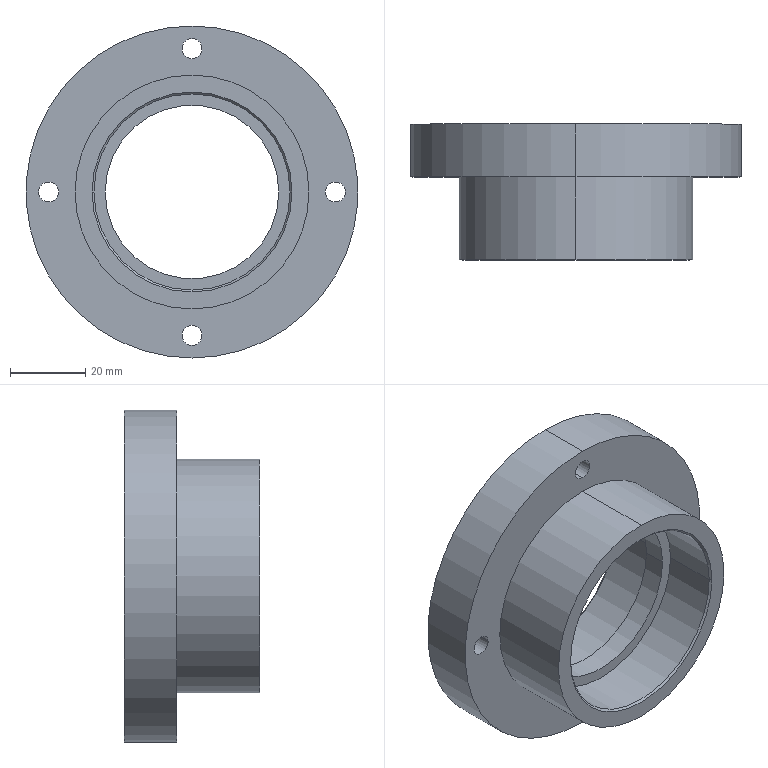Part | NX | 1 solid | 39 faces | box 88 x 36 x 88 mm | volume 75330 mm3 | cylinder 26 | plane 9 | cone 4 | commonest cylinder face diameters 5.3 x8 10 x6 52 x4 9.5 x2 46 x2 62 x2
STEP:
#1=CARTESIAN_POINT('',(0.,-14.,-44.));
#2=VERTEX_POINT('',#1);
#3=CARTESIAN_POINT('',(0.,-14.,44.));
#4=VERTEX_POINT('',#3);
#5=CARTESIAN_POINT('',(0.,-14.,0.));
#6=DIRECTION('',(0.,1.,0.));
#7=DIRECTION('',(0.,0.,1.));
#8=AXIS2_PLACEMENT_3D('',#5,#6,#7);
#9=CIRCLE('',#8,44.);
#10=EDGE_CURVE('',#2,#4,#9,.T.);
#11=ORIENTED_EDGE('',*,*,#10,.F.);
#12=CARTESIAN_POINT('',(0.,-14.,0.));
#13=DIRECTION('',(0.,1.,0.));
#14=DIRECTION('',(0.,0.,1.));
#15=AXIS2_PLACEMENT_3D('',#12,#13,#14);
#16=CIRCLE('',#15,44.);
#17=EDGE_CURVE('',#4,#2,#16,.T.);
#18=ORIENTED_EDGE('',*,*,#17,.F.);
#19=EDGE_LOOP('',(#11,#18));
#20=FACE_BOUND('',#19,.T.);
#21=CARTESIAN_POINT('',(0.,-14.,31.));
#22=VERTEX_POINT('',#21);
#23=CARTESIAN_POINT('',(0.,-14.,-31.));
#24=VERTEX_POINT('',#23);
#25=CARTESIAN_POINT('',(0.,-14.,0.));
#26=DIRECTION('',(0.,-1.,0.));
#27=DIRECTION('',(0.,0.,1.));
#28=AXIS2_PLACEMENT_3D('',#25,#26,#27);
#29=CIRCLE('',#28,31.);
#30=EDGE_CURVE('',#22,#24,#29,.T.);
#31=ORIENTED_EDGE('',*,*,#30,.F.);
#32=CARTESIAN_POINT('',(0.,-14.,0.));
#33=DIRECTION('',(0.,-1.,0.));
#34=DIRECTION('',(0.,0.,1.));
#35=AXIS2_PLACEMENT_3D('',#32,#33,#34);
#36=CIRCLE('',#35,31.);
#37=EDGE_CURVE('',#24,#22,#36,.T.);
#38=ORIENTED_EDGE('',*,*,#37,.F.);
#39=EDGE_LOOP('',(#31,#38));
#40=FACE_BOUND('',#39,.T.);
#41=CARTESIAN_POINT('',(40.65,-14.,0.));
#42=VERTEX_POINT('',#41);
#43=CARTESIAN_POINT('',(35.35,-14.,0.));
#44=VERTEX_POINT('',#43);
#45=CARTESIAN_POINT('',(38.,-14.,0.));
#46=DIRECTION('',(0.,-1.,0.));
#47=DIRECTION('',(1.,0.,0.));
#48=AXIS2_PLACEMENT_3D('',#45,#46,#47);
#49=CIRCLE('',#48,2.65);
#50=EDGE_CURVE('',#42,#44,#49,.T.);
#51=ORIENTED_EDGE('',*,*,#50,.F.);
#52=CARTESIAN_POINT('',(38.,-14.,0.));
#53=DIRECTION('',(0.,-1.,0.));
#54=DIRECTION('',(1.,0.,0.));
#55=AXIS2_PLACEMENT_3D('',#52,#53,#54);
#56=CIRCLE('',#55,2.65);
#57=EDGE_CURVE('',#44,#42,#56,.T.);
#58=ORIENTED_EDGE('',*,*,#57,.F.);
#59=EDGE_LOOP('',(#51,#58));
#60=FACE_BOUND('',#59,.T.);
#61=CARTESIAN_POINT('',(0.,-14.,-35.35));
#62=VERTEX_POINT('',#61);
#63=CARTESIAN_POINT('',(0.,-14.,-40.65));
#64=VERTEX_POINT('',#63);
#65=CARTESIAN_POINT('',(0.,-14.,-38.));
#66=DIRECTION('',(0.,-1.,0.));
#67=DIRECTION('',(0.,0.,-1.));
#68=AXIS2_PLACEMENT_3D('',#65,#66,#67);
#69=CIRCLE('',#68,2.65);
#70=EDGE_CURVE('',#62,#64,#69,.T.);
#71=ORIENTED_EDGE('',*,*,#70,.F.);
#72=CARTESIAN_POINT('',(0.,-14.,-38.));
#73=DIRECTION('',(0.,-1.,0.));
#74=DIRECTION('',(0.,0.,-1.));
#75=AXIS2_PLACEMENT_3D('',#72,#73,#74);
#76=CIRCLE('',#75,2.65);
#77=EDGE_CURVE('',#64,#62,#76,.T.);
#78=ORIENTED_EDGE('',*,*,#77,.F.);
#79=EDGE_LOOP('',(#71,#78));
#80=FACE_BOUND('',#79,.T.);
#81=CARTESIAN_POINT('',(-40.65,-14.,0.));
#82=VERTEX_POINT('',#81);
#83=CARTESIAN_POINT('',(-35.35,-14.,0.));
#84=VERTEX_POINT('',#83);
#85=CARTESIAN_POINT('',(-38.,-14.,0.));
#86=DIRECTION('',(0.,-1.,0.));
#87=DIRECTION('',(-1.,0.,0.));
#88=AXIS2_PLACEMENT_3D('',#85,#86,#87);
#89=CIRCLE('',#88,2.65);
#90=EDGE_CURVE('',#82,#84,#89,.T.);
#91=ORIENTED_EDGE('',*,*,#90,.F.);
#92=CARTESIAN_POINT('',(-38.,-14.,0.));
#93=DIRECTION('',(0.,-1.,0.));
#94=DIRECTION('',(-1.,0.,0.));
#95=AXIS2_PLACEMENT_3D('',#92,#93,#94);
#96=CIRCLE('',#95,2.65);
#97=EDGE_CURVE('',#84,#82,#96,.T.);
#98=ORIENTED_EDGE('',*,*,#97,.F.);
#99=EDGE_LOOP('',(#91,#98));
#100=FACE_BOUND('',#99,.T.);
#101=CARTESIAN_POINT('',(0.,-14.,35.35));
#102=VERTEX_POINT('',#101);
#103=CARTESIAN_POINT('',(0.,-14.,40.65));
#104=VERTEX_POINT('',#103);
#105=CARTESIAN_POINT('',(0.,-14.,38.));
#106=DIRECTION('',(0.,-1.,0.));
#107=DIRECTION('',(0.,0.,1.));
#108=AXIS2_PLACEMENT_3D('',#105,#106,#107);
#109=CIRCLE('',#108,2.65);
#110=EDGE_CURVE('',#102,#104,#109,.T.);
#111=ORIENTED_EDGE('',*,*,#110,.F.);
#112=CARTESIAN_POINT('',(0.,-14.,38.));
#113=DIRECTION('',(0.,-1.,0.));
#114=DIRECTION('',(0.,0.,1.));
#115=AXIS2_PLACEMENT_3D('',#112,#113,#114);
#116=CIRCLE('',#115,2.65);
#117=EDGE_CURVE('',#104,#102,#116,.T.);
#118=ORIENTED_EDGE('',*,*,#117,.F.);
#119=EDGE_LOOP('',(#111,#118));
#120=FACE_BOUND('',#119,.T.);
#121=CARTESIAN_POINT('',(0.,-14.,0.));
#122=DIRECTION('',(0.,1.,0.));
#123=DIRECTION('',(1.,0.,0.));
#124=AXIS2_PLACEMENT_3D('',#121,#122,#123);
#125=PLANE('',#124);
#126=ADVANCED_FACE('',(#20,#40,#60,#80,#100,#120),#125,.F.);
#127=CARTESIAN_POINT('',(0.,0.,-44.));
#128=VERTEX_POINT('',#127);
#129=CARTESIAN_POINT('',(0.,0.,44.));
#130=VERTEX_POINT('',#129);
#131=CARTESIAN_POINT('',(0.,0.,0.));
#132=DIRECTION('',(0.,-1.,0.));
#133=DIRECTION('',(0.,0.,1.));
#134=AXIS2_PLACEMENT_3D('',#131,#132,#133);
#135=CIRCLE('',#134,44.);
#136=EDGE_CURVE('',#128,#130,#135,.T.);
#137=ORIENTED_EDGE('',*,*,#136,.T.);
#138=CARTESIAN_POINT('',(0.,-37.8,44.));
#139=DIRECTION('',(0.,1.,0.));
#140=VECTOR('',#139,1000.);
#141=LINE('',#138,#140);
#142=EDGE_CURVE('',#4,#130,#141,.T.);
#143=ORIENTED_EDGE('',*,*,#142,.F.);
#144=ORIENTED_EDGE('',*,*,#17,.T.);
#145=CARTESIAN_POINT('',(0.,-37.8,-44.));
#146=DIRECTION('',(0.,1.,0.));
#147=VECTOR('',#146,1000.);
#148=LINE('',#145,#147);
#149=EDGE_CURVE('',#2,#128,#148,.T.);
#150=ORIENTED_EDGE('',*,*,#149,.T.);
#151=EDGE_LOOP('',(#137,#143,#144,#150));
#152=FACE_BOUND('',#151,.T.);
#153=CARTESIAN_POINT('',(0.,-37.8,0.));
#154=DIRECTION('',(0.,1.,0.));
#155=DIRECTION('',(0.,0.,-1.));
#156=AXIS2_PLACEMENT_3D('',#153,#154,#155);
#157=CYLINDRICAL_SURFACE('',#156,44.);
#158=ADVANCED_FACE('',(#152),#157,.T.);
#159=ORIENTED_EDGE('',*,*,#30,.T.);
#160=CARTESIAN_POINT('',(0.,-36.,-31.));
#161=VERTEX_POINT('',#160);
#162=CARTESIAN_POINT('',(0.,-37.8,-31.));
#163=DIRECTION('',(0.,1.,0.));
#164=VECTOR('',#163,1000.);
#165=LINE('',#162,#164);
#166=EDGE_CURVE('',#24,#161,#165,.F.);
#167=ORIENTED_EDGE('',*,*,#166,.T.);
#168=CARTESIAN_POINT('',(0.,-36.,31.));
#169=VERTEX_POINT('',#168);
#170=CARTESIAN_POINT('',(0.,-36.,0.));
#171=DIRECTION('',(0.,1.,0.));
#172=DIRECTION('',(0.,0.,1.));
#173=AXIS2_PLACEMENT_3D('',#170,#171,#172);
#174=CIRCLE('',#173,31.);
#175=EDGE_CURVE('',#161,#169,#174,.T.);
#176=ORIENTED_EDGE('',*,*,#175,.T.);
#177=CARTESIAN_POINT('',(0.,-37.8,31.));
#178=DIRECTION('',(0.,1.,0.));
#179=VECTOR('',#178,1000.);
#180=LINE('',#177,#179);
#181=EDGE_CURVE('',#22,#169,#180,.F.);
#182=ORIENTED_EDGE('',*,*,#181,.F.);
#183=EDGE_LOOP('',(#159,#167,#176,#182));
#184=FACE_BOUND('',#183,.T.);
#185=CARTESIAN_POINT('',(0.,-37.8,0.));
#186=DIRECTION('',(0.,1.,0.));
#187=DIRECTION('',(0.,0.,-1.));
#188=AXIS2_PLACEMENT_3D('',#185,#186,#187);
#189=CYLINDRICAL_SURFACE('',#188,31.);
#190=ADVANCED_FACE('',(#184),#189,.T.);
#191=ORIENTED_EDGE('',*,*,#136,.F.);
#192=CARTESIAN_POINT('',(0.,0.,0.));
#193=DIRECTION('',(0.,-1.,0.));
#194=DIRECTION('',(0.,0.,1.));
#195=AXIS2_PLACEMENT_3D('',#192,#193,#194);
#196=CIRCLE('',#195,44.);
#197=EDGE_CURVE('',#130,#128,#196,.T.);
#198=ORIENTED_EDGE('',*,*,#197,.F.);
#199=EDGE_LOOP('',(#191,#198));
#200=FACE_BOUND('',#199,.T.);
#201=CARTESIAN_POINT('',(33.25,0.,0.));
#202=VERTEX_POINT('',#201);
#203=CARTESIAN_POINT('',(42.75,0.,0.));
#204=VERTEX_POINT('',#203);
#205=CARTESIAN_POINT('',(38.,0.,0.));
#206=DIRECTION('',(0.,1.,0.));
#207=DIRECTION('',(-1.,0.,0.));
#208=AXIS2_PLACEMENT_3D('',#205,#206,#207);
#209=CIRCLE('',#208,4.75);
#210=EDGE_CURVE('',#202,#204,#209,.T.);
#211=ORIENTED_EDGE('',*,*,#210,.F.);
#212=CARTESIAN_POINT('',(38.,0.,0.));
#213=DIRECTION('',(0.,1.,0.));
#214=DIRECTION('',(-1.,0.,0.));
#215=AXIS2_PLACEMENT_3D('',#212,#213,#214);
#216=CIRCLE('',#215,4.75);
#217=EDGE_CURVE('',#204,#202,#216,.T.);
#218=ORIENTED_EDGE('',*,*,#217,.F.);
#219=EDGE_LOOP('',(#211,#218));
#220=FACE_BOUND('',#219,.T.);
#221=CARTESIAN_POINT('',(0.,0.,-33.));
#222=VERTEX_POINT('',#221);
#223=CARTESIAN_POINT('',(0.,0.,-43.));
#224=VERTEX_POINT('',#223);
#225=CARTESIAN_POINT('',(0.,0.,-38.));
#226=DIRECTION('',(0.,1.,0.));
#227=DIRECTION('',(0.,0.,1.));
#228=AXIS2_PLACEMENT_3D('',#225,#226,#227);
#229=CIRCLE('',#228,5.);
#230=EDGE_CURVE('',#222,#224,#229,.T.);
#231=ORIENTED_EDGE('',*,*,#230,.F.);
#232=CARTESIAN_POINT('',(0.,0.,-38.));
#233=DIRECTION('',(0.,1.,0.));
#234=DIRECTION('',(0.,0.,1.));
#235=AXIS2_PLACEMENT_3D('',#232,#233,#234);
#236=CIRCLE('',#235,5.);
#237=EDGE_CURVE('',#224,#222,#236,.T.);
#238=ORIENTED_EDGE('',*,*,#237,.F.);
#239=EDGE_LOOP('',(#231,#238));
#240=FACE_BOUND('',#239,.T.);
#241=CARTESIAN_POINT('',(-43.,0.,0.));
#242=VERTEX_POINT('',#241);
#243=CARTESIAN_POINT('',(-33.,0.,0.));
#244=VERTEX_POINT('',#243);
#245=CARTESIAN_POINT('',(-38.,0.,0.));
#246=DIRECTION('',(0.,1.,0.));
#247=DIRECTION('',(1.,0.,0.));
#248=AXIS2_PLACEMENT_3D('',#245,#246,#247);
#249=CIRCLE('',#248,5.);
#250=EDGE_CURVE('',#242,#244,#249,.T.);
#251=ORIENTED_EDGE('',*,*,#250,.F.);
#252=CARTESIAN_POINT('',(-38.,0.,0.));
#253=DIRECTION('',(0.,1.,0.));
#254=DIRECTION('',(1.,0.,0.));
#255=AXIS2_PLACEMENT_3D('',#252,#253,#254);
#256=CIRCLE('',#255,5.);
#257=EDGE_CURVE('',#244,#242,#256,.T.);
#258=ORIENTED_EDGE('',*,*,#257,.F.);
#259=EDGE_LOOP('',(#251,#258));
#260=FACE_BOUND('',#259,.T.);
#261=CARTESIAN_POINT('',(0.,0.,43.));
#262=VERTEX_POINT('',#261);
#263=CARTESIAN_POINT('',(0.,0.,33.));
#264=VERTEX_POINT('',#263);
#265=CARTESIAN_POINT('',(0.,0.,38.));
#266=DIRECTION('',(0.,1.,0.));
#267=DIRECTION('',(0.,0.,-1.));
#268=AXIS2_PLACEMENT_3D('',#265,#266,#267);
#269=CIRCLE('',#268,5.);
#270=EDGE_CURVE('',#262,#264,#269,.T.);
#271=ORIENTED_EDGE('',*,*,#270,.F.);
#272=CARTESIAN_POINT('',(0.,0.,38.));
#273=DIRECTION('',(0.,1.,0.));
#274=DIRECTION('',(0.,0.,-1.));
#275=AXIS2_PLACEMENT_3D('',#272,#273,#274);
#276=CIRCLE('',#275,5.);
#277=EDGE_CURVE('',#264,#262,#276,.T.);
#278=ORIENTED_EDGE('',*,*,#277,.F.);
#279=EDGE_LOOP('',(#271,#278));
#280=FACE_BOUND('',#279,.T.);
#281=CARTESIAN_POINT('',(26.5,0.,0.));
#282=VERTEX_POINT('',#281);
#283=CARTESIAN_POINT('',(-26.5,0.,0.));
#284=VERTEX_POINT('',#283);
#285=CARTESIAN_POINT('',(0.,0.,0.));
#286=DIRECTION('',(0.,1.,0.));
#287=DIRECTION('',(-1.,0.,0.));
#288=AXIS2_PLACEMENT_3D('',#285,#286,#287);
#289=CIRCLE('',#288,26.5);
#290=EDGE_CURVE('',#282,#284,#289,.T.);
#291=ORIENTED_EDGE('',*,*,#290,.F.);
#292=CARTESIAN_POINT('',(0.,0.,0.));
#293=DIRECTION('',(0.,1.,0.));
#294=DIRECTION('',(-1.,0.,0.));
#295=AXIS2_PLACEMENT_3D('',#292,#293,#294);
#296=CIRCLE('',#295,26.5);
#297=EDGE_CURVE('',#284,#282,#296,.T.);
#298=ORIENTED_EDGE('',*,*,#297,.F.);
#299=EDGE_LOOP('',(#291,#298));
#300=FACE_BOUND('',#299,.T.);
#301=CARTESIAN_POINT('',(0.,0.,0.));
#302=DIRECTION('',(0.,1.,0.));
#303=DIRECTION('',(1.,0.,0.));
#304=AXIS2_PLACEMENT_3D('',#301,#302,#303);
#305=PLANE('',#304);
#306=ADVANCED_FACE('',(#200,#220,#240,#260,#280,#300),#305,.T.);
#307=ORIENTED_EDGE('',*,*,#210,.T.);
#308=CARTESIAN_POINT('',(42.75,-5.4,0.));
#309=VERTEX_POINT('',#308);
#310=CARTESIAN_POINT('',(42.75,-41.525,0.));
#311=DIRECTION('',(0.,1.,0.));
#312=VECTOR('',#311,1000.);
#313=LINE('',#310,#312);
#314=EDGE_CURVE('',#309,#204,#313,.T.);
#315=ORIENTED_EDGE('',*,*,#314,.F.);
#316=CARTESIAN_POINT('',(33.25,-5.4,0.));
#317=VERTEX_POINT('',#316);
#318=CARTESIAN_POINT('',(38.,-5.4,0.));
#319=DIRECTION('',(0.,-1.,0.));
#320=DIRECTION('',(-1.,0.,0.));
#321=AXIS2_PLACEMENT_3D('',#318,#319,#320);
#322=CIRCLE('',#321,4.75);
#323=EDGE_CURVE('',#309,#317,#322,.T.);
#324=ORIENTED_EDGE('',*,*,#323,.T.);
#325=CARTESIAN_POINT('',(33.25,-41.525,0.));
#326=DIRECTION('',(0.,1.,0.));
#327=VECTOR('',#326,1000.);
#328=LINE('',#325,#327);
#329=EDGE_CURVE('',#317,#202,#328,.T.);
#330=ORIENTED_EDGE('',*,*,#329,.T.);
#331=EDGE_LOOP('',(#307,#315,#324,#330));
#332=FACE_BOUND('',#331,.T.);
#333=CARTESIAN_POINT('',(38.,-41.525,0.));
#334=DIRECTION('',(0.,1.,0.));
#335=DIRECTION('',(1.,0.,0.));
#336=AXIS2_PLACEMENT_3D('',#333,#334,#335);
#337=CYLINDRICAL_SURFACE('',#336,4.75);
#338=ADVANCED_FACE('',(#332),#337,.F.);
#339=ORIENTED_EDGE('',*,*,#175,.F.);
#340=CARTESIAN_POINT('',(0.,-36.,0.));
#341=DIRECTION('',(0.,1.,0.));
#342=DIRECTION('',(0.,0.,1.));
#343=AXIS2_PLACEMENT_3D('',#340,#341,#342);
#344=CIRCLE('',#343,31.);
#345=EDGE_CURVE('',#169,#161,#344,.T.);
#346=ORIENTED_EDGE('',*,*,#345,.F.);
#347=EDGE_LOOP('',(#339,#346));
#348=FACE_BOUND('',#347,.T.);
#349=CARTESIAN_POINT('',(-26.5,-36.,0.));
#350=VERTEX_POINT('',#349);
#351=CARTESIAN_POINT('',(26.5,-36.,0.));
#352=VERTEX_POINT('',#351);
#353=CARTESIAN_POINT('',(0.,-36.,0.));
#354=DIRECTION('',(0.,-1.,0.));
#355=DIRECTION('',(-1.,0.,0.));
#356=AXIS2_PLACEMENT_3D('',#353,#354,#355);
#357=CIRCLE('',#356,26.5);
#358=EDGE_CURVE('',#350,#352,#357,.T.);
#359=ORIENTED_EDGE('',*,*,#358,.F.);
#360=CARTESIAN_POINT('',(0.,-36.,0.));
#361=DIRECTION('',(0.,-1.,0.));
#362=DIRECTION('',(-1.,0.,0.));
#363=AXIS2_PLACEMENT_3D('',#360,#361,#362);
#364=CIRCLE('',#363,26.5);
#365=EDGE_CURVE('',#352,#350,#364,.T.);
#366=ORIENTED_EDGE('',*,*,#365,.F.);
#367=EDGE_LOOP('',(#359,#366));
#368=FACE_BOUND('',#367,.T.);
#369=CARTESIAN_POINT('',(0.,-36.,0.));
#370=DIRECTION('',(0.,1.,0.));
#371=DIRECTION('',(1.,0.,0.));
#372=AXIS2_PLACEMENT_3D('',#369,#370,#371);
#373=PLANE('',#372);
#374=ADVANCED_FACE('',(#348,#368),#373,.F.);
#375=CARTESIAN_POINT('',(38.,-5.4,0.));
#376=DIRECTION('',(0.,-1.,0.));
#377=DIRECTION('',(-1.,0.,0.));
#378=AXIS2_PLACEMENT_3D('',#375,#376,#377);
#379=CIRCLE('',#378,4.75);
#380=EDGE_CURVE('',#317,#309,#379,.T.);
#381=ORIENTED_EDGE('',*,*,#380,.F.);
#382=ORIENTED_EDGE('',*,*,#323,.F.);
#383=EDGE_LOOP('',(#381,#382));
#384=FACE_BOUND('',#383,.T.);
#385=CARTESIAN_POINT('',(40.65,-5.4,0.));
#386=VERTEX_POINT('',#385);
#387=CARTESIAN_POINT('',(35.35,-5.4,0.));
#388=VERTEX_POINT('',#387);
#389=CARTESIAN_POINT('',(38.,-5.4,0.));
#390=DIRECTION('',(0.,1.,0.));
#391=DIRECTION('',(1.,0.,0.));
#392=AXIS2_PLACEMENT_3D('',#389,#390,#391);
#393=CIRCLE('',#392,2.65);
#394=EDGE_CURVE('',#386,#388,#393,.T.);
#395=ORIENTED_EDGE('',*,*,#394,.F.);
#396=CARTESIAN_POINT('',(38.,-5.4,0.));
#397=DIRECTION('',(0.,1.,0.));
#398=DIRECTION('',(1.,0.,0.));
#399=AXIS2_PLACEMENT_3D('',#396,#397,#398);
#400=CIRCLE('',#399,2.65);
#401=EDGE_CURVE('',#388,#386,#400,.T.);
#402=ORIENTED_EDGE('',*,*,#401,.F.);
#403=EDGE_LOOP('',(#395,#402));
#404=FACE_BOUND('',#403,.T.);
#405=CARTESIAN_POINT('',(38.,-5.4,0.));
#406=DIRECTION('',(0.,1.,0.));
#407=DIRECTION('',(1.,0.,0.));
#408=AXIS2_PLACEMENT_3D('',#405,#406,#407);
#409=PLANE('',#408);
#410=ADVANCED_FACE('',(#384,#404),#409,.T.);
#411=ORIENTED_EDGE('',*,*,#50,.T.);
#412=CARTESIAN_POINT('',(35.35,-41.525,0.));
#413=DIRECTION('',(0.,1.,0.));
#414=VECTOR('',#413,1000.);
#415=LINE('',#412,#414);
#416=EDGE_CURVE('',#388,#44,#415,.F.);
#417=ORIENTED_EDGE('',*,*,#416,.F.);
#418=ORIENTED_EDGE('',*,*,#401,.T.);
#419=CARTESIAN_POINT('',(40.65,-41.525,0.));
#420=DIRECTION('',(0.,1.,0.));
#421=VECTOR('',#420,1000.);
#422=LINE('',#419,#421);
#423=EDGE_CURVE('',#386,#42,#422,.F.);
#424=ORIENTED_EDGE('',*,*,#423,.T.);
#425=EDGE_LOOP('',(#411,#417,#418,#424));
#426=FACE_BOUND('',#425,.T.);
#427=CARTESIAN_POINT('',(38.,-41.525,0.));
#428=DIRECTION('',(0.,1.,0.));
#429=DIRECTION('',(1.,0.,0.));
#430=AXIS2_PLACEMENT_3D('',#427,#428,#429);
#431=CYLINDRICAL_SURFACE('',#430,2.65);
#432=ADVANCED_FACE('',(#426),#431,.F.);
#433=CARTESIAN_POINT('',(-26.,-21.,0.));
#434=VERTEX_POINT('',#433);
#435=CARTESIAN_POINT('',(26.,-21.,0.));
#436=VERTEX_POINT('',#435);
#437=CARTESIAN_POINT('',(0.,-21.,0.));
#438=DIRECTION('',(0.,1.,0.));
#439=DIRECTION('',(-1.,0.,0.));
#440=AXIS2_PLACEMENT_3D('',#437,#438,#439);
#441=CIRCLE('',#440,26.);
#442=EDGE_CURVE('',#434,#436,#441,.T.);
#443=ORIENTED_EDGE('',*,*,#442,.F.);
#444=CARTESIAN_POINT('',(0.,-21.,0.));
#445=DIRECTION('',(0.,1.,0.));
#446=DIRECTION('',(-1.,0.,0.));
#447=AXIS2_PLACEMENT_3D('',#444,#445,#446);
#448=CIRCLE('',#447,26.);
#449=EDGE_CURVE('',#436,#434,#448,.T.);
#450=ORIENTED_EDGE('',*,*,#449,.F.);
#451=EDGE_LOOP('',(#443,#450));
#452=FACE_BOUND('',#451,.T.);
#453=CARTESIAN_POINT('',(23.,-21.,0.));
#454=VERTEX_POINT('',#453);
#455=CARTESIAN_POINT('',(-23.,-21.,0.));
#456=VERTEX_POINT('',#455);
#457=CARTESIAN_POINT('',(0.,-21.,0.));
#458=DIRECTION('',(0.,-1.,0.));
#459=DIRECTION('',(1.,0.,0.));
#460=AXIS2_PLACEMENT_3D('',#457,#458,#459);
#461=CIRCLE('',#460,23.);
#462=EDGE_CURVE('',#454,#456,#461,.T.);
#463=ORIENTED_EDGE('',*,*,#462,.F.);
#464=CARTESIAN_POINT('',(0.,-21.,0.));
#465=DIRECTION('',(0.,-1.,0.));
#466=DIRECTION('',(1.,0.,0.));
#467=AXIS2_PLACEMENT_3D('',#464,#465,#466);
#468=CIRCLE('',#467,23.);
#469=EDGE_CURVE('',#456,#454,#468,.T.);
#470=ORIENTED_EDGE('',*,*,#469,.F.);
#471=EDGE_LOOP('',(#463,#470));
#472=FACE_BOUND('',#471,.T.);
#473=CARTESIAN_POINT('',(0.,-21.,0.));
#474=DIRECTION('',(0.,-1.,0.));
#475=DIRECTION('',(0.,0.,-1.));
#476=AXIS2_PLACEMENT_3D('',#473,#474,#475);
#477=PLANE('',#476);
#478=ADVANCED_FACE('',(#452,#472),#477,.T.);
#479=ORIENTED_EDGE('',*,*,#230,.T.);
#480=CARTESIAN_POINT('',(0.,-6.,-43.));
#481=VERTEX_POINT('',#480);
#482=CARTESIAN_POINT('',(0.,-41.58,-43.));
#483=DIRECTION('',(0.,1.,0.));
#484=VECTOR('',#483,1000.);
#485=LINE('',#482,#484);
#486=EDGE_CURVE('',#224,#481,#485,.F.);
#487=ORIENTED_EDGE('',*,*,#486,.T.);
#488=CARTESIAN_POINT('',(0.,-6.,-33.));
#489=VERTEX_POINT('',#488);
#490=CARTESIAN_POINT('',(0.,-6.,-38.));
#491=DIRECTION('',(0.,-1.,0.));
#492=DIRECTION('',(0.,0.,-1.));
#493=AXIS2_PLACEMENT_3D('',#490,#491,#492);
#494=CIRCLE('',#493,5.);
#495=EDGE_CURVE('',#481,#489,#494,.T.);
#496=ORIENTED_EDGE('',*,*,#495,.T.);
#497=CARTESIAN_POINT('',(0.,-41.58,-33.));
#498=DIRECTION('',(0.,1.,0.));
#499=VECTOR('',#498,1000.);
#500=LINE('',#497,#499);
#501=EDGE_CURVE('',#222,#489,#500,.F.);
#502=ORIENTED_EDGE('',*,*,#501,.F.);
#503=EDGE_LOOP('',(#479,#487,#496,#502));
#504=FACE_BOUND('',#503,.T.);
#505=CARTESIAN_POINT('',(0.,-41.58,-38.));
#506=DIRECTION('',(0.,1.,0.));
#507=DIRECTION('',(0.,0.,-1.));
#508=AXIS2_PLACEMENT_3D('',#505,#506,#507);
#509=CYLINDRICAL_SURFACE('',#508,5.);
#510=ADVANCED_FACE('',(#504),#509,.F.);
#511=ORIENTED_EDGE('',*,*,#462,.T.);
#512=CARTESIAN_POINT('',(-23.,-15.,0.));
#513=VERTEX_POINT('',#512);
#514=CARTESIAN_POINT('',(-23.,-15.,0.));
#515=DIRECTION('',(0.,-1.,0.));
#516=VECTOR('',#515,1000.);
#517=LINE('',#514,#516);
#518=EDGE_CURVE('',#456,#513,#517,.F.);
#519=ORIENTED_EDGE('',*,*,#518,.T.);
#520=CARTESIAN_POINT('',(23.,-15.,0.));
#521=VERTEX_POINT('',#520);
#522=CARTESIAN_POINT('',(0.,-15.,0.));
#523=DIRECTION('',(0.,1.,0.));
#524=DIRECTION('',(1.,0.,0.));
#525=AXIS2_PLACEMENT_3D('',#522,#523,#524);
#526=CIRCLE('',#525,23.);
#527=EDGE_CURVE('',#513,#521,#526,.T.);
#528=ORIENTED_EDGE('',*,*,#527,.T.);
#529=CARTESIAN_POINT('',(23.,-15.,0.));
#530=DIRECTION('',(0.,-1.,0.));
#531=VECTOR('',#530,1000.);
#532=LINE('',#529,#531);
#533=EDGE_CURVE('',#454,#521,#532,.F.);
#534=ORIENTED_EDGE('',*,*,#533,.F.);
#535=EDGE_LOOP('',(#511,#519,#528,#534));
#536=FACE_BOUND('',#535,.T.);
#537=CARTESIAN_POINT('',(0.,-15.,0.));
#538=DIRECTION('',(0.,-1.,0.));
#539=DIRECTION('',(-1.,0.,0.));
#540=AXIS2_PLACEMENT_3D('',#537,#538,#539);
#541=CYLINDRICAL_SURFACE('',#540,23.);
#542=ADVANCED_FACE('',(#536),#541,.F.);
#543=ORIENTED_EDGE('',*,*,#495,.F.);
#544=CARTESIAN_POINT('',(0.,-6.,-38.));
#545=DIRECTION('',(0.,-1.,0.));
#546=DIRECTION('',(0.,0.,-1.));
#547=AXIS2_PLACEMENT_3D('',#544,#545,#546);
#548=CIRCLE('',#547,5.);
#549=EDGE_CURVE('',#489,#481,#548,.T.);
#550=ORIENTED_EDGE('',*,*,#549,.F.);
#551=EDGE_LOOP('',(#543,#550));
#552=FACE_BOUND('',#551,.T.);
#553=CARTESIAN_POINT('',(0.,-6.,-35.35));
#554=VERTEX_POINT('',#553);
#555=CARTESIAN_POINT('',(0.,-6.,-40.65));
#556=VERTEX_POINT('',#555);
#557=CARTESIAN_POINT('',(0.,-6.,-38.));
#558=DIRECTION('',(0.,1.,0.));
#559=DIRECTION('',(0.,0.,-1.));
#560=AXIS2_PLACEMENT_3D('',#557,#558,#559);
#561=CIRCLE('',#560,2.65);
#562=EDGE_CURVE('',#554,#556,#561,.T.);
#563=ORIENTED_EDGE('',*,*,#562,.F.);
#564=CARTESIAN_POINT('',(0.,-6.,-38.));
#565=DIRECTION('',(0.,1.,0.));
#566=DIRECTION('',(0.,0.,-1.));
#567=AXIS2_PLACEMENT_3D('',#564,#565,#566);
#568=CIRCLE('',#567,2.65);
#569=EDGE_CURVE('',#556,#554,#568,.T.);
#570=ORIENTED_EDGE('',*,*,#569,.F.);
#571=EDGE_LOOP('',(#563,#570));
#572=FACE_BOUND('',#571,.T.);
#573=CARTESIAN_POINT('',(0.,-6.,-38.));
#574=DIRECTION('',(0.,1.,0.));
#575=DIRECTION('',(1.,0.,0.));
#576=AXIS2_PLACEMENT_3D('',#573,#574,#575);
#577=PLANE('',#576);
#578=ADVANCED_FACE('',(#552,#572),#577,.T.);
#579=ORIENTED_EDGE('',*,*,#70,.T.);
#580=CARTESIAN_POINT('',(0.,-41.58,-40.65));
#581=DIRECTION('',(0.,1.,0.));
#582=VECTOR('',#581,1000.);
#583=LINE('',#580,#582);
#584=EDGE_CURVE('',#556,#64,#583,.F.);
#585=ORIENTED_EDGE('',*,*,#584,.F.);
#586=ORIENTED_EDGE('',*,*,#569,.T.);
#587=CARTESIAN_POINT('',(0.,-41.58,-35.35));
#588=DIRECTION('',(0.,1.,0.));
#589=VECTOR('',#588,1000.);
#590=LINE('',#587,#589);
#591=EDGE_CURVE('',#554,#62,#590,.F.);
#592=ORIENTED_EDGE('',*,*,#591,.T.);
#593=EDGE_LOOP('',(#579,#585,#586,#592));
#594=FACE_BOUND('',#593,.T.);
#595=CARTESIAN_POINT('',(0.,-41.58,-38.));
#596=DIRECTION('',(0.,1.,0.));
#597=DIRECTION('',(0.,0.,-1.));
#598=AXIS2_PLACEMENT_3D('',#595,#596,#597);
#599=CYLINDRICAL_SURFACE('',#598,2.65);
#600=ADVANCED_FACE('',(#594),#599,.F.);
#601=CARTESIAN_POINT('',(-26.,-35.5,0.));
#602=VERTEX_POINT('',#601);
#603=CARTESIAN_POINT('',(26.,-35.5,0.));
#604=VERTEX_POINT('',#603);
#605=CARTESIAN_POINT('',(0.,-35.5,0.));
#606=DIRECTION('',(0.,-1.,0.));
#607=DIRECTION('',(1.,0.,0.));
#608=AXIS2_PLACEMENT_3D('',#605,#606,#607);
#609=CIRCLE('',#608,26.);
#610=EDGE_CURVE('',#602,#604,#609,.T.);
#611=ORIENTED_EDGE('',*,*,#610,.F.);
#612=CARTESIAN_POINT('',(-26.25,-35.75,0.));
#613=DIRECTION('',(-0.7071,-0.7071,0.));
#614=VECTOR('',#613,1000.);
#615=LINE('',#612,#614);
#616=EDGE_CURVE('',#350,#602,#615,.F.);
#617=ORIENTED_EDGE('',*,*,#616,.F.);
#618=ORIENTED_EDGE('',*,*,#358,.T.);
#619=CARTESIAN_POINT('',(26.25,-35.75,0.));
#620=DIRECTION('',(0.7071,-0.7071,0.));
#621=VECTOR('',#620,1000.);
#622=LINE('',#619,#621);
#623=EDGE_CURVE('',#352,#604,#622,.F.);
#624=ORIENTED_EDGE('',*,*,#623,.T.);
#625=EDGE_LOOP('',(#611,#617,#618,#624));
#626=FACE_BOUND('',#625,.T.);
#627=CARTESIAN_POINT('',(0.,-35.75,0.));
#628=DIRECTION('',(0.,-1.,0.));
#629=DIRECTION('',(-1.,0.,0.));
#630=AXIS2_PLACEMENT_3D('',#627,#628,#629);
#631=CONICAL_SURFACE('',#630,26.25,0.7854);
#632=ADVANCED_FACE('',(#626),#631,.F.);
#633=CARTESIAN_POINT('',(-33.,-6.,0.));
#634=VERTEX_POINT('',#633);
#635=CARTESIAN_POINT('',(-43.,-6.,0.));
#636=VERTEX_POINT('',#635);
#637=CARTESIAN_POINT('',(-38.,-6.,0.));
#638=DIRECTION('',(0.,-1.,0.));
#639=DIRECTION('',(1.,0.,0.));
#640=AXIS2_PLACEMENT_3D('',#637,#638,#639);
#641=CIRCLE('',#640,5.);
#642=EDGE_CURVE('',#634,#636,#641,.T.);
#643=ORIENTED_EDGE('',*,*,#642,.T.);
#644=CARTESIAN_POINT('',(-43.,-41.58,0.));
#645=DIRECTION('',(0.,1.,0.));
#646=VECTOR('',#645,1000.);
#647=LINE('',#644,#646);
#648=EDGE_CURVE('',#242,#636,#647,.F.);
#649=ORIENTED_EDGE('',*,*,#648,.F.);
#650=ORIENTED_EDGE('',*,*,#250,.T.);
#651=CARTESIAN_POINT('',(-33.,-41.58,0.));
#652=DIRECTION('',(0.,1.,0.));
#653=VECTOR('',#652,1000.);
#654=LINE('',#651,#653);
#655=EDGE_CURVE('',#244,#634,#654,.F.);
#656=ORIENTED_EDGE('',*,*,#655,.T.);
#657=EDGE_LOOP('',(#643,#649,#650,#656));
#658=FACE_BOUND('',#657,.T.);
#659=CARTESIAN_POINT('',(-38.,-41.58,0.));
#660=DIRECTION('',(0.,1.,0.));
#661=DIRECTION('',(-1.,0.,0.));
#662=AXIS2_PLACEMENT_3D('',#659,#660,#661);
#663=CYLINDRICAL_SURFACE('',#662,5.);
#664=ADVANCED_FACE('',(#658),#663,.F.);
#665=ORIENTED_EDGE('',*,*,#290,.T.);
#666=CARTESIAN_POINT('',(-26.,-0.5,0.));
#667=VERTEX_POINT('',#666);
#668=CARTESIAN_POINT('',(-26.25,-0.25,0.));
#669=DIRECTION('',(-0.7071,0.7071,0.));
#670=VECTOR('',#669,1000.);
#671=LINE('',#668,#670);
#672=EDGE_CURVE('',#284,#667,#671,.F.);
#673=ORIENTED_EDGE('',*,*,#672,.T.);
#674=CARTESIAN_POINT('',(26.,-0.5,0.));
#675=VERTEX_POINT('',#674);
#676=CARTESIAN_POINT('',(0.,-0.5,0.));
#677=DIRECTION('',(0.,1.,0.));
#678=DIRECTION('',(1.,0.,0.));
#679=AXIS2_PLACEMENT_3D('',#676,#677,#678);
#680=CIRCLE('',#679,26.);
#681=EDGE_CURVE('',#675,#667,#680,.T.);
#682=ORIENTED_EDGE('',*,*,#681,.F.);
#683=CARTESIAN_POINT('',(26.25,-0.25,0.));
#684=DIRECTION('',(0.7071,0.7071,0.));
#685=VECTOR('',#684,1000.);
#686=LINE('',#683,#685);
#687=EDGE_CURVE('',#282,#675,#686,.F.);
#688=ORIENTED_EDGE('',*,*,#687,.F.);
#689=EDGE_LOOP('',(#665,#673,#682,#688));
#690=FACE_BOUND('',#689,.T.);
#691=CARTESIAN_POINT('',(0.,-0.25,0.));
#692=DIRECTION('',(0.,1.,0.));
#693=DIRECTION('',(1.,0.,0.));
#694=AXIS2_PLACEMENT_3D('',#691,#692,#693);
#695=CONICAL_SURFACE('',#694,26.25,0.7854);
#696=ADVANCED_FACE('',(#690),#695,.F.);
#697=ORIENTED_EDGE('',*,*,#642,.F.);
#698=CARTESIAN_POINT('',(-38.,-6.,0.));
#699=DIRECTION('',(0.,-1.,0.));
#700=DIRECTION('',(1.,0.,0.));
#701=AXIS2_PLACEMENT_3D('',#698,#699,#700);
#702=CIRCLE('',#701,5.);
#703=EDGE_CURVE('',#636,#634,#702,.T.);
#704=ORIENTED_EDGE('',*,*,#703,.F.);
#705=EDGE_LOOP('',(#697,#704));
#706=FACE_BOUND('',#705,.T.);
#707=CARTESIAN_POINT('',(-40.65,-6.,0.));
#708=VERTEX_POINT('',#707);
#709=CARTESIAN_POINT('',(-35.35,-6.,0.));
#710=VERTEX_POINT('',#709);
#711=CARTESIAN_POINT('',(-38.,-6.,0.));
#712=DIRECTION('',(0.,1.,0.));
#713=DIRECTION('',(-1.,0.,0.));
#714=AXIS2_PLACEMENT_3D('',#711,#712,#713);
#715=CIRCLE('',#714,2.65);
#716=EDGE_CURVE('',#708,#710,#715,.T.);
#717=ORIENTED_EDGE('',*,*,#716,.F.);
#718=CARTESIAN_POINT('',(-38.,-6.,0.));
#719=DIRECTION('',(0.,1.,0.));
#720=DIRECTION('',(-1.,0.,0.));
#721=AXIS2_PLACEMENT_3D('',#718,#719,#720);
#722=CIRCLE('',#721,2.65);
#723=EDGE_CURVE('',#710,#708,#722,.T.);
#724=ORIENTED_EDGE('',*,*,#723,.F.);
#725=EDGE_LOOP('',(#717,#724));
#726=FACE_BOUND('',#725,.T.);
#727=CARTESIAN_POINT('',(-38.,-6.,0.));
#728=DIRECTION('',(0.,1.,0.));
#729=DIRECTION('',(1.,0.,0.));
#730=AXIS2_PLACEMENT_3D('',#727,#728,#729);
#731=PLANE('',#730);
#732=ADVANCED_FACE('',(#706,#726),#731,.T.);
#733=ORIENTED_EDGE('',*,*,#716,.T.);
#734=CARTESIAN_POINT('',(-35.35,-41.58,0.));
#735=DIRECTION('',(0.,1.,0.));
#736=VECTOR('',#735,1000.);
#737=LINE('',#734,#736);
#738=EDGE_CURVE('',#84,#710,#737,.T.);
#739=ORIENTED_EDGE('',*,*,#738,.F.);
#740=ORIENTED_EDGE('',*,*,#97,.T.);
#741=CARTESIAN_POINT('',(-40.65,-41.58,0.));
#742=DIRECTION('',(0.,1.,0.));
#743=VECTOR('',#742,1000.);
#744=LINE('',#741,#743);
#745=EDGE_CURVE('',#82,#708,#744,.T.);
#746=ORIENTED_EDGE('',*,*,#745,.T.);
#747=EDGE_LOOP('',(#733,#739,#740,#746));
#748=FACE_BOUND('',#747,.T.);
#749=CARTESIAN_POINT('',(-38.,-41.58,0.));
#750=DIRECTION('',(0.,1.,0.));
#751=DIRECTION('',(-1.,0.,0.));
#752=AXIS2_PLACEMENT_3D('',#749,#750,#751);
#753=CYLINDRICAL_SURFACE('',#752,2.65);
#754=ADVANCED_FACE('',(#748),#753,.F.);
#755=ORIENTED_EDGE('',*,*,#442,.T.);
#756=CARTESIAN_POINT('',(26.,0.,0.));
#757=DIRECTION('',(0.,1.,0.));
#758=VECTOR('',#757,1000.);
#759=LINE('',#756,#758);
#760=EDGE_CURVE('',#604,#436,#759,.T.);
#761=ORIENTED_EDGE('',*,*,#760,.F.);
#762=CARTESIAN_POINT('',(0.,-35.5,0.));
#763=DIRECTION('',(0.,-1.,0.));
#764=DIRECTION('',(1.,0.,0.));
#765=AXIS2_PLACEMENT_3D('',#762,#763,#764);
#766=CIRCLE('',#765,26.);
#767=EDGE_CURVE('',#604,#602,#766,.T.);
#768=ORIENTED_EDGE('',*,*,#767,.T.);
#769=CARTESIAN_POINT('',(-26.,0.,0.));
#770=DIRECTION('',(0.,1.,0.));
#771=VECTOR('',#770,1000.);
#772=LINE('',#769,#771);
#773=EDGE_CURVE('',#602,#434,#772,.T.);
#774=ORIENTED_EDGE('',*,*,#773,.T.);
#775=EDGE_LOOP('',(#755,#761,#768,#774));
#776=FACE_BOUND('',#775,.T.);
#777=CARTESIAN_POINT('',(0.,0.,0.));
#778=DIRECTION('',(0.,1.,0.));
#779=DIRECTION('',(1.,0.,0.));
#780=AXIS2_PLACEMENT_3D('',#777,#778,#779);
#781=CYLINDRICAL_SURFACE('',#780,26.);
#782=ADVANCED_FACE('',(#776),#781,.F.);
#783=ORIENTED_EDGE('',*,*,#270,.T.);
#784=CARTESIAN_POINT('',(0.,-6.,33.));
#785=VERTEX_POINT('',#784);
#786=CARTESIAN_POINT('',(0.,-41.58,33.));
#787=DIRECTION('',(0.,1.,0.));
#788=VECTOR('',#787,1000.);
#789=LINE('',#786,#788);
#790=EDGE_CURVE('',#264,#785,#789,.F.);
#791=ORIENTED_EDGE('',*,*,#790,.T.);
#792=CARTESIAN_POINT('',(0.,-6.,43.));
#793=VERTEX_POINT('',#792);
#794=CARTESIAN_POINT('',(0.,-6.,38.));
#795=DIRECTION('',(0.,-1.,0.));
#796=DIRECTION('',(0.,0.,1.));
#797=AXIS2_PLACEMENT_3D('',#794,#795,#796);
#798=CIRCLE('',#797,5.);
#799=EDGE_CURVE('',#785,#793,#798,.T.);
#800=ORIENTED_EDGE('',*,*,#799,.T.);
#801=CARTESIAN_POINT('',(0.,-41.58,43.));
#802=DIRECTION('',(0.,1.,0.));
#803=VECTOR('',#802,1000.);
#804=LINE('',#801,#803);
#805=EDGE_CURVE('',#262,#793,#804,.F.);
#806=ORIENTED_EDGE('',*,*,#805,.F.);
#807=EDGE_LOOP('',(#783,#791,#800,#806));
#808=FACE_BOUND('',#807,.T.);
#809=CARTESIAN_POINT('',(0.,-41.58,38.));
#810=DIRECTION('',(0.,1.,0.));
#811=DIRECTION('',(0.,0.,1.));
#812=AXIS2_PLACEMENT_3D('',#809,#810,#811);
#813=CYLINDRICAL_SURFACE('',#812,5.);
#814=ADVANCED_FACE('',(#808),#813,.F.);
#815=CARTESIAN_POINT('',(-26.,-15.,0.));
#816=VERTEX_POINT('',#815);
#817=CARTESIAN_POINT('',(26.,-15.,0.));
#818=VERTEX_POINT('',#817);
#819=CARTESIAN_POINT('',(0.,-15.,0.));
#820=DIRECTION('',(0.,-1.,0.));
#821=DIRECTION('',(-1.,0.,0.));
#822=AXIS2_PLACEMENT_3D('',#819,#820,#821);
#823=CIRCLE('',#822,26.);
#824=EDGE_CURVE('',#816,#818,#823,.T.);
#825=ORIENTED_EDGE('',*,*,#824,.F.);
#826=CARTESIAN_POINT('',(0.,-15.,0.));
#827=DIRECTION('',(0.,-1.,0.));
#828=DIRECTION('',(-1.,0.,0.));
#829=AXIS2_PLACEMENT_3D('',#826,#827,#828);
#830=CIRCLE('',#829,26.);
#831=EDGE_CURVE('',#818,#816,#830,.T.);
#832=ORIENTED_EDGE('',*,*,#831,.F.);
#833=EDGE_LOOP('',(#825,#832));
#834=FACE_BOUND('',#833,.T.);
#835=CARTESIAN_POINT('',(0.,-15.,0.));
#836=DIRECTION('',(0.,1.,0.));
#837=DIRECTION('',(1.,0.,0.));
#838=AXIS2_PLACEMENT_3D('',#835,#836,#837);
#839=CIRCLE('',#838,23.);
#840=EDGE_CURVE('',#521,#513,#839,.T.);
#841=ORIENTED_EDGE('',*,*,#840,.F.);
#842=ORIENTED_EDGE('',*,*,#527,.F.);
#843=EDGE_LOOP('',(#841,#842));
#844=FACE_BOUND('',#843,.T.);
#845=CARTESIAN_POINT('',(0.,-15.,0.));
#846=DIRECTION('',(0.,-1.,0.));
#847=DIRECTION('',(0.,0.,-1.));
#848=AXIS2_PLACEMENT_3D('',#845,#846,#847);
#849=PLANE('',#848);
#850=ADVANCED_FACE('',(#834,#844),#849,.F.);
#851=CARTESIAN_POINT('',(0.,-6.,38.));
#852=DIRECTION('',(0.,-1.,0.));
#853=DIRECTION('',(0.,0.,1.));
#854=AXIS2_PLACEMENT_3D('',#851,#852,#853);
#855=CIRCLE('',#854,5.);
#856=EDGE_CURVE('',#793,#785,#855,.T.);
#857=ORIENTED_EDGE('',*,*,#856,.F.);
#858=ORIENTED_EDGE('',*,*,#799,.F.);
#859=EDGE_LOOP('',(#857,#858));
#860=FACE_BOUND('',#859,.T.);
#861=CARTESIAN_POINT('',(0.,-6.,40.65));
#862=VERTEX_POINT('',#861);
#863=CARTESIAN_POINT('',(0.,-6.,35.35));
#864=VERTEX_POINT('',#863);
#865=CARTESIAN_POINT('',(0.,-6.,38.));
#866=DIRECTION('',(0.,1.,0.));
#867=DIRECTION('',(0.,0.,1.));
#868=AXIS2_PLACEMENT_3D('',#865,#866,#867);
#869=CIRCLE('',#868,2.65);
#870=EDGE_CURVE('',#862,#864,#869,.T.);
#871=ORIENTED_EDGE('',*,*,#870,.F.);
#872=CARTESIAN_POINT('',(0.,-6.,38.));
#873=DIRECTION('',(0.,1.,0.));
#874=DIRECTION('',(0.,0.,1.));
#875=AXIS2_PLACEMENT_3D('',#872,#873,#874);
#876=CIRCLE('',#875,2.65);
#877=EDGE_CURVE('',#864,#862,#876,.T.);
#878=ORIENTED_EDGE('',*,*,#877,.F.);
#879=EDGE_LOOP('',(#871,#878));
#880=FACE_BOUND('',#879,.T.);
#881=CARTESIAN_POINT('',(0.,-6.,38.));
#882=DIRECTION('',(0.,1.,0.));
#883=DIRECTION('',(1.,0.,0.));
#884=AXIS2_PLACEMENT_3D('',#881,#882,#883);
#885=PLANE('',#884);
#886=ADVANCED_FACE('',(#860,#880),#885,.T.);
#887=ORIENTED_EDGE('',*,*,#110,.T.);
#888=CARTESIAN_POINT('',(0.,-41.58,40.65));
#889=DIRECTION('',(0.,1.,0.));
#890=VECTOR('',#889,1000.);
#891=LINE('',#888,#890);
#892=EDGE_CURVE('',#104,#862,#891,.T.);
#893=ORIENTED_EDGE('',*,*,#892,.T.);
#894=ORIENTED_EDGE('',*,*,#870,.T.);
#895=CARTESIAN_POINT('',(0.,-41.58,35.35));
#896=DIRECTION('',(0.,1.,0.));
#897=VECTOR('',#896,1000.);
#898=LINE('',#895,#897);
#899=EDGE_CURVE('',#102,#864,#898,.T.);
#900=ORIENTED_EDGE('',*,*,#899,.F.);
#901=EDGE_LOOP('',(#887,#893,#894,#900));
#902=FACE_BOUND('',#901,.T.);
#903=CARTESIAN_POINT('',(0.,-41.58,38.));
#904=DIRECTION('',(0.,1.,0.));
#905=DIRECTION('',(0.,0.,1.));
#906=AXIS2_PLACEMENT_3D('',#903,#904,#905);
#907=CYLINDRICAL_SURFACE('',#906,2.65);
#908=ADVANCED_FACE('',(#902),#907,.F.);
#909=CARTESIAN_POINT('',(0.,-0.5,0.));
#910=DIRECTION('',(0.,1.,0.));
#911=DIRECTION('',(1.,0.,0.));
#912=AXIS2_PLACEMENT_3D('',#909,#910,#911);
#913=CIRCLE('',#912,26.);
#914=EDGE_CURVE('',#667,#675,#913,.T.);
#915=ORIENTED_EDGE('',*,*,#914,.T.);
#916=CARTESIAN_POINT('',(26.,0.,0.));
#917=DIRECTION('',(0.,1.,0.));
#918=VECTOR('',#917,1000.);
#919=LINE('',#916,#918);
#920=EDGE_CURVE('',#818,#675,#919,.T.);
#921=ORIENTED_EDGE('',*,*,#920,.F.);
#922=ORIENTED_EDGE('',*,*,#831,.T.);
#923=CARTESIAN_POINT('',(-26.,0.,0.));
#924=DIRECTION('',(0.,1.,0.));
#925=VECTOR('',#924,1000.);
#926=LINE('',#923,#925);
#927=EDGE_CURVE('',#816,#667,#926,.T.);
#928=ORIENTED_EDGE('',*,*,#927,.T.);
#929=EDGE_LOOP('',(#915,#921,#922,#928));
#930=FACE_BOUND('',#929,.T.);
#931=CARTESIAN_POINT('',(0.,0.,0.));
#932=DIRECTION('',(0.,1.,0.));
#933=DIRECTION('',(1.,0.,0.));
#934=AXIS2_PLACEMENT_3D('',#931,#932,#933);
#935=CYLINDRICAL_SURFACE('',#934,26.);
#936=ADVANCED_FACE('',(#930),#935,.F.);
#937=ORIENTED_EDGE('',*,*,#380,.T.);
#938=ORIENTED_EDGE('',*,*,#314,.T.);
#939=ORIENTED_EDGE('',*,*,#217,.T.);
#940=ORIENTED_EDGE('',*,*,#329,.F.);
#941=EDGE_LOOP('',(#937,#938,#939,#940));
#942=FACE_BOUND('',#941,.T.);
#943=CARTESIAN_POINT('',(38.,-41.525,0.));
#944=DIRECTION('',(0.,1.,0.));
#945=DIRECTION('',(1.,0.,0.));
#946=AXIS2_PLACEMENT_3D('',#943,#944,#945);
#947=CYLINDRICAL_SURFACE('',#946,4.75);
#948=ADVANCED_FACE('',(#942),#947,.F.);
#949=ORIENTED_EDGE('',*,*,#824,.T.);
#950=ORIENTED_EDGE('',*,*,#920,.T.);
#951=ORIENTED_EDGE('',*,*,#681,.T.);
#952=ORIENTED_EDGE('',*,*,#927,.F.);
#953=EDGE_LOOP('',(#949,#950,#951,#952));
#954=FACE_BOUND('',#953,.T.);
#955=CARTESIAN_POINT('',(0.,0.,0.));
#956=DIRECTION('',(0.,1.,0.));
#957=DIRECTION('',(1.,0.,0.));
#958=AXIS2_PLACEMENT_3D('',#955,#956,#957);
#959=CYLINDRICAL_SURFACE('',#958,26.);
#960=ADVANCED_FACE('',(#954),#959,.F.);
#961=ORIENTED_EDGE('',*,*,#166,.F.);
#962=ORIENTED_EDGE('',*,*,#37,.T.);
#963=ORIENTED_EDGE('',*,*,#181,.T.);
#964=ORIENTED_EDGE('',*,*,#345,.T.);
#965=EDGE_LOOP('',(#961,#962,#963,#964));
#966=FACE_BOUND('',#965,.T.);
#967=CARTESIAN_POINT('',(0.,-37.8,0.));
#968=DIRECTION('',(0.,1.,0.));
#969=DIRECTION('',(0.,0.,-1.));
#970=AXIS2_PLACEMENT_3D('',#967,#968,#969);
#971=CYLINDRICAL_SURFACE('',#970,31.);
#972=ADVANCED_FACE('',(#966),#971,.T.);
#973=ORIENTED_EDGE('',*,*,#610,.T.);
#974=ORIENTED_EDGE('',*,*,#760,.T.);
#975=ORIENTED_EDGE('',*,*,#449,.T.);
#976=ORIENTED_EDGE('',*,*,#773,.F.);
#977=EDGE_LOOP('',(#973,#974,#975,#976));
#978=FACE_BOUND('',#977,.T.);
#979=CARTESIAN_POINT('',(0.,0.,0.));
#980=DIRECTION('',(0.,1.,0.));
#981=DIRECTION('',(1.,0.,0.));
#982=AXIS2_PLACEMENT_3D('',#979,#980,#981);
#983=CYLINDRICAL_SURFACE('',#982,26.);
#984=ADVANCED_FACE('',(#978),#983,.F.);
#985=ORIENTED_EDGE('',*,*,#10,.T.);
#986=ORIENTED_EDGE('',*,*,#142,.T.);
#987=ORIENTED_EDGE('',*,*,#197,.T.);
#988=ORIENTED_EDGE('',*,*,#149,.F.);
#989=EDGE_LOOP('',(#985,#986,#987,#988));
#990=FACE_BOUND('',#989,.T.);
#991=CARTESIAN_POINT('',(0.,-37.8,0.));
#992=DIRECTION('',(0.,1.,0.));
#993=DIRECTION('',(0.,0.,-1.));
#994=AXIS2_PLACEMENT_3D('',#991,#992,#993);
#995=CYLINDRICAL_SURFACE('',#994,44.);
#996=ADVANCED_FACE('',(#990),#995,.T.);
#997=ORIENTED_EDGE('',*,*,#892,.F.);
#998=ORIENTED_EDGE('',*,*,#117,.T.);
#999=ORIENTED_EDGE('',*,*,#899,.T.);
#1000=ORIENTED_EDGE('',*,*,#877,.T.);
#1001=EDGE_LOOP('',(#997,#998,#999,#1000));
#1002=FACE_BOUND('',#1001,.T.);
#1003=CARTESIAN_POINT('',(0.,-41.58,38.));
#1004=DIRECTION('',(0.,1.,0.));
#1005=DIRECTION('',(0.,0.,1.));
#1006=AXIS2_PLACEMENT_3D('',#1003,#1004,#1005);
#1007=CYLINDRICAL_SURFACE('',#1006,2.65);
#1008=ADVANCED_FACE('',(#1002),#1007,.F.);
#1009=ORIENTED_EDGE('',*,*,#90,.T.);
#1010=ORIENTED_EDGE('',*,*,#738,.T.);
#1011=ORIENTED_EDGE('',*,*,#723,.T.);
#1012=ORIENTED_EDGE('',*,*,#745,.F.);
#1013=EDGE_LOOP('',(#1009,#1010,#1011,#1012));
#1014=FACE_BOUND('',#1013,.T.);
#1015=CARTESIAN_POINT('',(-38.,-41.58,0.));
#1016=DIRECTION('',(0.,1.,0.));
#1017=DIRECTION('',(-1.,0.,0.));
#1018=AXIS2_PLACEMENT_3D('',#1015,#1016,#1017);
#1019=CYLINDRICAL_SURFACE('',#1018,2.65);
#1020=ADVANCED_FACE('',(#1014),#1019,.F.);
#1021=ORIENTED_EDGE('',*,*,#562,.T.);
#1022=ORIENTED_EDGE('',*,*,#584,.T.);
#1023=ORIENTED_EDGE('',*,*,#77,.T.);
#1024=ORIENTED_EDGE('',*,*,#591,.F.);
#1025=EDGE_LOOP('',(#1021,#1022,#1023,#1024));
#1026=FACE_BOUND('',#1025,.T.);
#1027=CARTESIAN_POINT('',(0.,-41.58,-38.));
#1028=DIRECTION('',(0.,1.,0.));
#1029=DIRECTION('',(0.,0.,-1.));
#1030=AXIS2_PLACEMENT_3D('',#1027,#1028,#1029);
#1031=CYLINDRICAL_SURFACE('',#1030,2.65);
#1032=ADVANCED_FACE('',(#1026),#1031,.F.);
#1033=ORIENTED_EDGE('',*,*,#394,.T.);
#1034=ORIENTED_EDGE('',*,*,#416,.T.);
#1035=ORIENTED_EDGE('',*,*,#57,.T.);
#1036=ORIENTED_EDGE('',*,*,#423,.F.);
#1037=EDGE_LOOP('',(#1033,#1034,#1035,#1036));
#1038=FACE_BOUND('',#1037,.T.);
#1039=CARTESIAN_POINT('',(38.,-41.525,0.));
#1040=DIRECTION('',(0.,1.,0.));
#1041=DIRECTION('',(1.,0.,0.));
#1042=AXIS2_PLACEMENT_3D('',#1039,#1040,#1041);
#1043=CYLINDRICAL_SURFACE('',#1042,2.65);
#1044=ADVANCED_FACE('',(#1038),#1043,.F.);
#1045=ORIENTED_EDGE('',*,*,#616,.T.);
#1046=ORIENTED_EDGE('',*,*,#767,.F.);
#1047=ORIENTED_EDGE('',*,*,#623,.F.);
#1048=ORIENTED_EDGE('',*,*,#365,.T.);
#1049=EDGE_LOOP('',(#1045,#1046,#1047,#1048));
#1050=FACE_BOUND('',#1049,.T.);
#1051=CARTESIAN_POINT('',(0.,-35.75,0.));
#1052=DIRECTION('',(0.,-1.,0.));
#1053=DIRECTION('',(-1.,0.,0.));
#1054=AXIS2_PLACEMENT_3D('',#1051,#1052,#1053);
#1055=CONICAL_SURFACE('',#1054,26.25,0.7854);
#1056=ADVANCED_FACE('',(#1050),#1055,.F.);
#1057=ORIENTED_EDGE('',*,*,#840,.T.);
#1058=ORIENTED_EDGE('',*,*,#518,.F.);
#1059=ORIENTED_EDGE('',*,*,#469,.T.);
#1060=ORIENTED_EDGE('',*,*,#533,.T.);
#1061=EDGE_LOOP('',(#1057,#1058,#1059,#1060));
#1062=FACE_BOUND('',#1061,.T.);
#1063=CARTESIAN_POINT('',(0.,-15.,0.));
#1064=DIRECTION('',(0.,-1.,0.));
#1065=DIRECTION('',(-1.,0.,0.));
#1066=AXIS2_PLACEMENT_3D('',#1063,#1064,#1065);
#1067=CYLINDRICAL_SURFACE('',#1066,23.);
#1068=ADVANCED_FACE('',(#1062),#1067,.F.);
#1069=ORIENTED_EDGE('',*,*,#914,.F.);
#1070=ORIENTED_EDGE('',*,*,#672,.F.);
#1071=ORIENTED_EDGE('',*,*,#297,.T.);
#1072=ORIENTED_EDGE('',*,*,#687,.T.);
#1073=EDGE_LOOP('',(#1069,#1070,#1071,#1072));
#1074=FACE_BOUND('',#1073,.T.);
#1075=CARTESIAN_POINT('',(0.,-0.25,0.));
#1076=DIRECTION('',(0.,1.,0.));
#1077=DIRECTION('',(1.,0.,0.));
#1078=AXIS2_PLACEMENT_3D('',#1075,#1076,#1077);
#1079=CONICAL_SURFACE('',#1078,26.25,0.7854);
#1080=ADVANCED_FACE('',(#1074),#1079,.F.);
#1081=ORIENTED_EDGE('',*,*,#856,.T.);
#1082=ORIENTED_EDGE('',*,*,#790,.F.);
#1083=ORIENTED_EDGE('',*,*,#277,.T.);
#1084=ORIENTED_EDGE('',*,*,#805,.T.);
#1085=EDGE_LOOP('',(#1081,#1082,#1083,#1084));
#1086=FACE_BOUND('',#1085,.T.);
#1087=CARTESIAN_POINT('',(0.,-41.58,38.));
#1088=DIRECTION('',(0.,1.,0.));
#1089=DIRECTION('',(0.,0.,1.));
#1090=AXIS2_PLACEMENT_3D('',#1087,#1088,#1089);
#1091=CYLINDRICAL_SURFACE('',#1090,5.);
#1092=ADVANCED_FACE('',(#1086),#1091,.F.);
#1093=ORIENTED_EDGE('',*,*,#648,.T.);
#1094=ORIENTED_EDGE('',*,*,#703,.T.);
#1095=ORIENTED_EDGE('',*,*,#655,.F.);
#1096=ORIENTED_EDGE('',*,*,#257,.T.);
#1097=EDGE_LOOP('',(#1093,#1094,#1095,#1096));
#1098=FACE_BOUND('',#1097,.T.);
#1099=CARTESIAN_POINT('',(-38.,-41.58,0.));
#1100=DIRECTION('',(0.,1.,0.));
#1101=DIRECTION('',(-1.,0.,0.));
#1102=AXIS2_PLACEMENT_3D('',#1099,#1100,#1101);
#1103=CYLINDRICAL_SURFACE('',#1102,5.);
#1104=ADVANCED_FACE('',(#1098),#1103,.F.);
#1105=ORIENTED_EDGE('',*,*,#486,.F.);
#1106=ORIENTED_EDGE('',*,*,#237,.T.);
#1107=ORIENTED_EDGE('',*,*,#501,.T.);
#1108=ORIENTED_EDGE('',*,*,#549,.T.);
#1109=EDGE_LOOP('',(#1105,#1106,#1107,#1108));
#1110=FACE_BOUND('',#1109,.T.);
#1111=CARTESIAN_POINT('',(0.,-41.58,-38.));
#1112=DIRECTION('',(0.,1.,0.));
#1113=DIRECTION('',(0.,0.,-1.));
#1114=AXIS2_PLACEMENT_3D('',#1111,#1112,#1113);
#1115=CYLINDRICAL_SURFACE('',#1114,5.);
#1116=ADVANCED_FACE('',(#1110),#1115,.F.);
#1117=CLOSED_SHELL('',(#126,#158,#190,#306,#338,#374,#410,#432,#478,#510,#542,#578,#600,#632,#664,#696,#732,#754,#782,#814,#850,#886,#908,#936,#948,#960,#972,#984,#996,#1008,#1020,#1032,#1044,#1056,#1068,#1080,#1092,#1104,#1116));
#1118=MANIFOLD_SOLID_BREP('',#1117);
#1119=(LENGTH_UNIT()NAMED_UNIT(*)SI_UNIT(.MILLI.,.METRE.));
#1120=UNCERTAINTY_MEASURE_WITH_UNIT(LENGTH_MEASURE(0.00001),#1119,'','');
#1121=(NAMED_UNIT(*)PLANE_ANGLE_UNIT()SI_UNIT($,.RADIAN.));
#1122=(NAMED_UNIT(*)SI_UNIT($,.STERADIAN.)SOLID_ANGLE_UNIT());
#1123=(GEOMETRIC_REPRESENTATION_CONTEXT(3)GLOBAL_UNCERTAINTY_ASSIGNED_CONTEXT((#1120))GLOBAL_UNIT_ASSIGNED_CONTEXT((#1119,#1121,#1122))REPRESENTATION_CONTEXT('',''));
#1124=ADVANCED_BREP_SHAPE_REPRESENTATION('',(#1118),#1123);